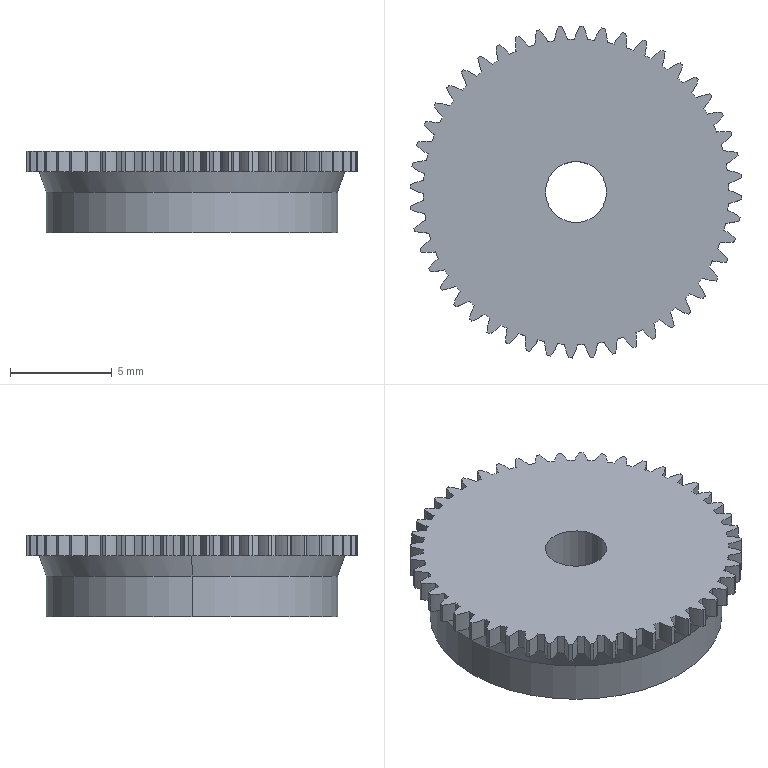Part | SolidWorks | features ICE 2, Blend 1, CirPattern 1, Cut 1, Extrusion 1 | 1 solid | 252 faces | box 16.296 x 16.296 x 4 mm | volume 653.065 mm3 | cylinder 200 | plane 50 | cone 2 | commonest cylinder face diameters 5.301 x100 15 x48 16.3 x48 3 x2 14.32 x2